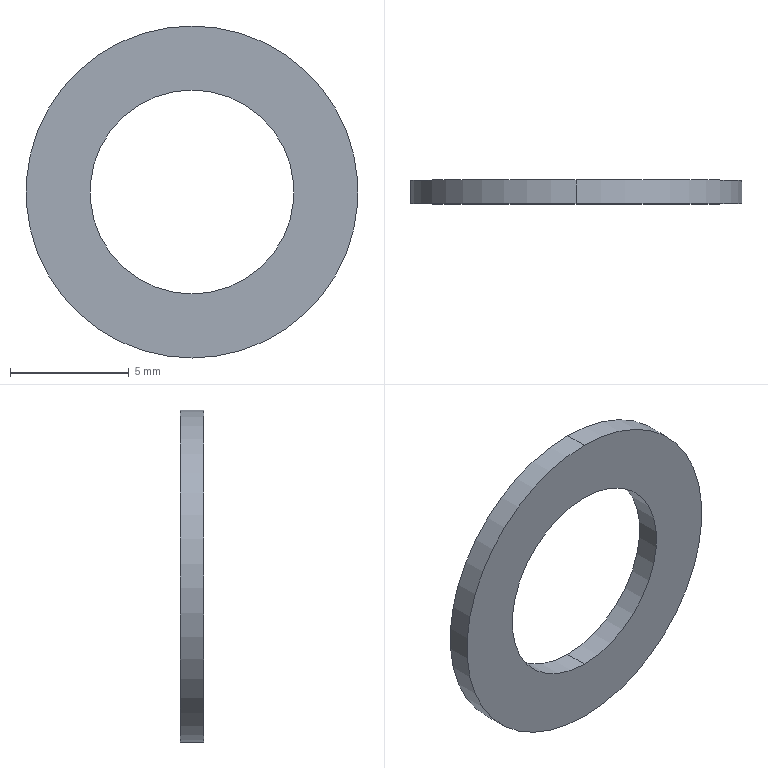Part | STEP file | Vibration plate 3-06_default | 1 solid | 6 faces | box 14 x 1 x 14 mm | volume 95.85 mm3 | cylinder 4 | plane 2 | commonest cylinder face diameters 8.6 x2 14 x2
STEP:
#1=CARTESIAN_POINT('',(0.,0.,0.));
#2=DIRECTION('',(0.,0.,1.));
#3=DIRECTION('',(1.,0.,0.));
#4=AXIS2_PLACEMENT_3D('',#1,#2,#3);
#5=CARTESIAN_POINT('',(0.,0.,4.3));
#6=VERTEX_POINT('',#5);
#7=CARTESIAN_POINT('',(0.,1.,4.3));
#8=VERTEX_POINT('',#7);
#9=CARTESIAN_POINT('',(0.,0.,4.3));
#10=DIRECTION('',(0.,1.,0.));
#11=VECTOR('',#10,1.);
#12=LINE('',#9,#11);
#13=CARTESIAN_POINT('',(0.,0.,0.));
#14=DIRECTION('',(0.,1.,0.));
#15=DIRECTION('',(0.,0.,1.));
#16=AXIS2_PLACEMENT_3D('',#13,#14,#15);
#17=CYLINDRICAL_SURFACE('',#16,4.3);
#18=CARTESIAN_POINT('',(6.283,0.));
#19=DIRECTION('',(0.,1.));
#20=VECTOR('',#19,1.);
#21=LINE('',#18,#20);
#22=(GEOMETRIC_REPRESENTATION_CONTEXT(2)PARAMETRIC_REPRESENTATION_CONTEXT()REPRESENTATION_CONTEXT('',''));
#23=DEFINITIONAL_REPRESENTATION('',(#21),#22);
#24=PCURVE('',#17,#23);
#25=CARTESIAN_POINT('',(0.,0.,0.));
#26=DIRECTION('',(0.,1.,0.));
#27=DIRECTION('',(0.,0.,1.));
#28=AXIS2_PLACEMENT_3D('',#25,#26,#27);
#29=CYLINDRICAL_SURFACE('',#28,4.3);
#30=CARTESIAN_POINT('',(0.,0.));
#31=DIRECTION('',(0.,1.));
#32=VECTOR('',#31,1.);
#33=LINE('',#30,#32);
#34=(GEOMETRIC_REPRESENTATION_CONTEXT(2)PARAMETRIC_REPRESENTATION_CONTEXT()REPRESENTATION_CONTEXT('',''));
#35=DEFINITIONAL_REPRESENTATION('',(#33),#34);
#36=PCURVE('',#29,#35);
#37=SURFACE_CURVE('',#12,(#24,#36),.PCURVE_S1.);
#38=EDGE_CURVE('',#6,#8,#37,.T.);
#39=ORIENTED_EDGE('',*,*,#38,.T.);
#40=CARTESIAN_POINT('',(0.,1.,-4.3));
#41=VERTEX_POINT('',#40);
#42=CARTESIAN_POINT('',(0.,1.,0.));
#43=DIRECTION('',(0.,-1.,0.));
#44=DIRECTION('',(0.,0.,1.));
#45=AXIS2_PLACEMENT_3D('',#42,#43,#44);
#46=CIRCLE('',#45,4.3);
#47=CARTESIAN_POINT('',(6.283,1.));
#48=DIRECTION('',(-1.,0.));
#49=VECTOR('',#48,1.);
#50=LINE('',#47,#49);
#51=(GEOMETRIC_REPRESENTATION_CONTEXT(2)PARAMETRIC_REPRESENTATION_CONTEXT()REPRESENTATION_CONTEXT('',''));
#52=DEFINITIONAL_REPRESENTATION('',(#50),#51);
#53=PCURVE('',#17,#52);
#54=CARTESIAN_POINT('',(0.,1.,0.));
#55=DIRECTION('',(0.,1.,0.));
#56=DIRECTION('',(0.,0.,1.));
#57=AXIS2_PLACEMENT_3D('',#54,#55,#56);
#58=PLANE('',#57);
#59=CARTESIAN_POINT('',(4.3,0.));
#60=CARTESIAN_POINT('',(4.3,-7.448));
#61=CARTESIAN_POINT('',(-2.15,-3.724));
#62=CARTESIAN_POINT('',(-8.6,0.));
#63=CARTESIAN_POINT('',(-2.15,3.724));
#64=CARTESIAN_POINT('',(4.3,7.448));
#65=CARTESIAN_POINT('',(4.3,0.));
#66=(BOUNDED_CURVE()B_SPLINE_CURVE(2,(#59,#60,#61,#62,#63,#64,#65),.UNSPECIFIED.,.T.,.F.)B_SPLINE_CURVE_WITH_KNOTS((1,2,2,2,2,1),(-2.094,0.,2.094,4.189,6.283,8.378),.UNSPECIFIED.)CURVE()GEOMETRIC_REPRESENTATION_ITEM()RATIONAL_B_SPLINE_CURVE((1.,0.5,1.,0.5,1.,0.5,1.))REPRESENTATION_ITEM(''));
#67=(GEOMETRIC_REPRESENTATION_CONTEXT(2)PARAMETRIC_REPRESENTATION_CONTEXT()REPRESENTATION_CONTEXT('',''));
#68=DEFINITIONAL_REPRESENTATION('',(#66),#67);
#69=PCURVE('',#58,#68);
#70=SURFACE_CURVE('',#46,(#53,#69),.PCURVE_S1.);
#71=EDGE_CURVE('',#8,#41,#70,.T.);
#72=ORIENTED_EDGE('',*,*,#71,.T.);
#73=CARTESIAN_POINT('',(0.,0.,-4.3));
#74=VERTEX_POINT('',#73);
#75=CARTESIAN_POINT('',(0.,0.,-4.3));
#76=DIRECTION('',(0.,1.,0.));
#77=VECTOR('',#76,1.);
#78=LINE('',#75,#77);
#79=CARTESIAN_POINT('',(3.142,0.));
#80=DIRECTION('',(0.,1.));
#81=VECTOR('',#80,1.);
#82=LINE('',#79,#81);
#83=(GEOMETRIC_REPRESENTATION_CONTEXT(2)PARAMETRIC_REPRESENTATION_CONTEXT()REPRESENTATION_CONTEXT('',''));
#84=DEFINITIONAL_REPRESENTATION('',(#82),#83);
#85=PCURVE('',#17,#84);
#86=CARTESIAN_POINT('',(3.142,0.));
#87=DIRECTION('',(0.,1.));
#88=VECTOR('',#87,1.);
#89=LINE('',#86,#88);
#90=(GEOMETRIC_REPRESENTATION_CONTEXT(2)PARAMETRIC_REPRESENTATION_CONTEXT()REPRESENTATION_CONTEXT('',''));
#91=DEFINITIONAL_REPRESENTATION('',(#89),#90);
#92=PCURVE('',#29,#91);
#93=SURFACE_CURVE('',#78,(#85,#92),.PCURVE_S1.);
#94=EDGE_CURVE('',#74,#41,#93,.T.);
#95=ORIENTED_EDGE('',*,*,#94,.F.);
#96=CARTESIAN_POINT('',(0.,0.,0.));
#97=DIRECTION('',(0.,-1.,0.));
#98=DIRECTION('',(0.,0.,1.));
#99=AXIS2_PLACEMENT_3D('',#96,#97,#98);
#100=CIRCLE('',#99,4.3);
#101=CARTESIAN_POINT('',(6.283,0.));
#102=DIRECTION('',(-1.,0.));
#103=VECTOR('',#102,1.);
#104=LINE('',#101,#103);
#105=(GEOMETRIC_REPRESENTATION_CONTEXT(2)PARAMETRIC_REPRESENTATION_CONTEXT()REPRESENTATION_CONTEXT('',''));
#106=DEFINITIONAL_REPRESENTATION('',(#104),#105);
#107=PCURVE('',#17,#106);
#108=CARTESIAN_POINT('',(0.,0.,0.));
#109=DIRECTION('',(0.,1.,0.));
#110=DIRECTION('',(0.,0.,1.));
#111=AXIS2_PLACEMENT_3D('',#108,#109,#110);
#112=PLANE('',#111);
#113=CARTESIAN_POINT('',(4.3,0.));
#114=CARTESIAN_POINT('',(4.3,-7.448));
#115=CARTESIAN_POINT('',(-2.15,-3.724));
#116=CARTESIAN_POINT('',(-8.6,0.));
#117=CARTESIAN_POINT('',(-2.15,3.724));
#118=CARTESIAN_POINT('',(4.3,7.448));
#119=CARTESIAN_POINT('',(4.3,0.));
#120=(BOUNDED_CURVE()B_SPLINE_CURVE(2,(#113,#114,#115,#116,#117,#118,#119),.UNSPECIFIED.,.T.,.F.)B_SPLINE_CURVE_WITH_KNOTS((1,2,2,2,2,1),(-2.094,0.,2.094,4.189,6.283,8.378),.UNSPECIFIED.)CURVE()GEOMETRIC_REPRESENTATION_ITEM()RATIONAL_B_SPLINE_CURVE((1.,0.5,1.,0.5,1.,0.5,1.))REPRESENTATION_ITEM(''));
#121=(GEOMETRIC_REPRESENTATION_CONTEXT(2)PARAMETRIC_REPRESENTATION_CONTEXT()REPRESENTATION_CONTEXT('',''));
#122=DEFINITIONAL_REPRESENTATION('',(#120),#121);
#123=PCURVE('',#112,#122);
#124=SURFACE_CURVE('',#100,(#107,#123),.PCURVE_S1.);
#125=EDGE_CURVE('',#6,#74,#124,.T.);
#126=ORIENTED_EDGE('',*,*,#125,.F.);
#127=EDGE_LOOP('',(#39,#72,#95,#126));
#128=FACE_BOUND('',#127,.F.);
#129=ADVANCED_FACE('',(#128),#17,.F.);
#130=CARTESIAN_POINT('',(0.,0.,7.));
#131=VERTEX_POINT('',#130);
#132=CARTESIAN_POINT('',(0.,0.,-7.));
#133=VERTEX_POINT('',#132);
#134=CARTESIAN_POINT('',(0.,0.,0.));
#135=DIRECTION('',(0.,1.,0.));
#136=DIRECTION('',(0.,0.,1.));
#137=AXIS2_PLACEMENT_3D('',#134,#135,#136);
#138=CIRCLE('',#137,7.);
#139=CARTESIAN_POINT('',(0.,0.,0.));
#140=DIRECTION('',(0.,1.,0.));
#141=DIRECTION('',(0.,0.,1.));
#142=AXIS2_PLACEMENT_3D('',#139,#140,#141);
#143=CYLINDRICAL_SURFACE('',#142,7.);
#144=CARTESIAN_POINT('',(0.,0.));
#145=DIRECTION('',(1.,0.));
#146=VECTOR('',#145,1.);
#147=LINE('',#144,#146);
#148=(GEOMETRIC_REPRESENTATION_CONTEXT(2)PARAMETRIC_REPRESENTATION_CONTEXT()REPRESENTATION_CONTEXT('',''));
#149=DEFINITIONAL_REPRESENTATION('',(#147),#148);
#150=PCURVE('',#143,#149);
#151=CARTESIAN_POINT('',(0.,0.));
#152=DIRECTION('',(1.,0.));
#153=AXIS2_PLACEMENT_2D('',#151,#152);
#154=CIRCLE('',#153,7.);
#155=(GEOMETRIC_REPRESENTATION_CONTEXT(2)PARAMETRIC_REPRESENTATION_CONTEXT()REPRESENTATION_CONTEXT('',''));
#156=DEFINITIONAL_REPRESENTATION('',(#154),#155);
#157=PCURVE('',#112,#156);
#158=SURFACE_CURVE('',#138,(#150,#157),.PCURVE_S1.);
#159=EDGE_CURVE('',#131,#133,#158,.T.);
#160=ORIENTED_EDGE('',*,*,#159,.T.);
#161=CARTESIAN_POINT('',(0.,1.,-7.));
#162=VERTEX_POINT('',#161);
#163=CARTESIAN_POINT('',(0.,0.,-7.));
#164=DIRECTION('',(0.,1.,0.));
#165=VECTOR('',#164,1.);
#166=LINE('',#163,#165);
#167=CARTESIAN_POINT('',(3.142,0.));
#168=DIRECTION('',(0.,1.));
#169=VECTOR('',#168,1.);
#170=LINE('',#167,#169);
#171=(GEOMETRIC_REPRESENTATION_CONTEXT(2)PARAMETRIC_REPRESENTATION_CONTEXT()REPRESENTATION_CONTEXT('',''));
#172=DEFINITIONAL_REPRESENTATION('',(#170),#171);
#173=PCURVE('',#143,#172);
#174=CARTESIAN_POINT('',(0.,0.,0.));
#175=DIRECTION('',(0.,1.,0.));
#176=DIRECTION('',(0.,0.,1.));
#177=AXIS2_PLACEMENT_3D('',#174,#175,#176);
#178=CYLINDRICAL_SURFACE('',#177,7.);
#179=CARTESIAN_POINT('',(3.142,0.));
#180=DIRECTION('',(0.,1.));
#181=VECTOR('',#180,1.);
#182=LINE('',#179,#181);
#183=(GEOMETRIC_REPRESENTATION_CONTEXT(2)PARAMETRIC_REPRESENTATION_CONTEXT()REPRESENTATION_CONTEXT('',''));
#184=DEFINITIONAL_REPRESENTATION('',(#182),#183);
#185=PCURVE('',#178,#184);
#186=SURFACE_CURVE('',#166,(#173,#185),.PCURVE_S1.);
#187=EDGE_CURVE('',#133,#162,#186,.T.);
#188=ORIENTED_EDGE('',*,*,#187,.T.);
#189=CARTESIAN_POINT('',(0.,1.,7.));
#190=VERTEX_POINT('',#189);
#191=CARTESIAN_POINT('',(0.,1.,0.));
#192=DIRECTION('',(0.,-1.,0.));
#193=DIRECTION('',(0.,0.,1.));
#194=AXIS2_PLACEMENT_3D('',#191,#192,#193);
#195=CIRCLE('',#194,7.);
#196=CARTESIAN_POINT('',(6.283,1.));
#197=DIRECTION('',(-1.,0.));
#198=VECTOR('',#197,1.);
#199=LINE('',#196,#198);
#200=(GEOMETRIC_REPRESENTATION_CONTEXT(2)PARAMETRIC_REPRESENTATION_CONTEXT()REPRESENTATION_CONTEXT('',''));
#201=DEFINITIONAL_REPRESENTATION('',(#199),#200);
#202=PCURVE('',#143,#201);
#203=CARTESIAN_POINT('',(7.,0.));
#204=CARTESIAN_POINT('',(7.,-12.124));
#205=CARTESIAN_POINT('',(-3.5,-6.062));
#206=CARTESIAN_POINT('',(-14.,0.));
#207=CARTESIAN_POINT('',(-3.5,6.062));
#208=CARTESIAN_POINT('',(7.,12.124));
#209=CARTESIAN_POINT('',(7.,0.));
#210=(BOUNDED_CURVE()B_SPLINE_CURVE(2,(#203,#204,#205,#206,#207,#208,#209),.UNSPECIFIED.,.T.,.F.)B_SPLINE_CURVE_WITH_KNOTS((1,2,2,2,2,1),(-2.094,0.,2.094,4.189,6.283,8.378),.UNSPECIFIED.)CURVE()GEOMETRIC_REPRESENTATION_ITEM()RATIONAL_B_SPLINE_CURVE((1.,0.5,1.,0.5,1.,0.5,1.))REPRESENTATION_ITEM(''));
#211=(GEOMETRIC_REPRESENTATION_CONTEXT(2)PARAMETRIC_REPRESENTATION_CONTEXT()REPRESENTATION_CONTEXT('',''));
#212=DEFINITIONAL_REPRESENTATION('',(#210),#211);
#213=PCURVE('',#58,#212);
#214=SURFACE_CURVE('',#195,(#202,#213),.PCURVE_S1.);
#215=EDGE_CURVE('',#162,#190,#214,.T.);
#216=ORIENTED_EDGE('',*,*,#215,.T.);
#217=CARTESIAN_POINT('',(0.,0.,7.));
#218=DIRECTION('',(0.,1.,0.));
#219=VECTOR('',#218,1.);
#220=LINE('',#217,#219);
#221=CARTESIAN_POINT('',(0.,0.));
#222=DIRECTION('',(0.,1.));
#223=VECTOR('',#222,1.);
#224=LINE('',#221,#223);
#225=(GEOMETRIC_REPRESENTATION_CONTEXT(2)PARAMETRIC_REPRESENTATION_CONTEXT()REPRESENTATION_CONTEXT('',''));
#226=DEFINITIONAL_REPRESENTATION('',(#224),#225);
#227=PCURVE('',#143,#226);
#228=CARTESIAN_POINT('',(6.283,0.));
#229=DIRECTION('',(0.,1.));
#230=VECTOR('',#229,1.);
#231=LINE('',#228,#230);
#232=(GEOMETRIC_REPRESENTATION_CONTEXT(2)PARAMETRIC_REPRESENTATION_CONTEXT()REPRESENTATION_CONTEXT('',''));
#233=DEFINITIONAL_REPRESENTATION('',(#231),#232);
#234=PCURVE('',#178,#233);
#235=SURFACE_CURVE('',#220,(#227,#234),.PCURVE_S1.);
#236=EDGE_CURVE('',#131,#190,#235,.T.);
#237=ORIENTED_EDGE('',*,*,#236,.F.);
#238=EDGE_LOOP('',(#160,#188,#216,#237));
#239=FACE_BOUND('',#238,.T.);
#240=ADVANCED_FACE('',(#239),#143,.T.);
#241=ORIENTED_EDGE('',*,*,#125,.F.);
#242=CARTESIAN_POINT('',(0.,0.,0.));
#243=DIRECTION('',(0.,-1.,0.));
#244=DIRECTION('',(0.,0.,1.));
#245=AXIS2_PLACEMENT_3D('',#242,#243,#244);
#246=CIRCLE('',#245,4.3);
#247=CARTESIAN_POINT('',(4.3,0.));
#248=CARTESIAN_POINT('',(4.3,-7.448));
#249=CARTESIAN_POINT('',(-2.15,-3.724));
#250=CARTESIAN_POINT('',(-8.6,0.));
#251=CARTESIAN_POINT('',(-2.15,3.724));
#252=CARTESIAN_POINT('',(4.3,7.448));
#253=CARTESIAN_POINT('',(4.3,0.));
#254=(BOUNDED_CURVE()B_SPLINE_CURVE(2,(#247,#248,#249,#250,#251,#252,#253),.UNSPECIFIED.,.T.,.F.)B_SPLINE_CURVE_WITH_KNOTS((1,2,2,2,2,1),(-2.094,0.,2.094,4.189,6.283,8.378),.UNSPECIFIED.)CURVE()GEOMETRIC_REPRESENTATION_ITEM()RATIONAL_B_SPLINE_CURVE((1.,0.5,1.,0.5,1.,0.5,1.))REPRESENTATION_ITEM(''));
#255=(GEOMETRIC_REPRESENTATION_CONTEXT(2)PARAMETRIC_REPRESENTATION_CONTEXT()REPRESENTATION_CONTEXT('',''));
#256=DEFINITIONAL_REPRESENTATION('',(#254),#255);
#257=PCURVE('',#112,#256);
#258=CARTESIAN_POINT('',(6.283,0.));
#259=DIRECTION('',(-1.,0.));
#260=VECTOR('',#259,1.);
#261=LINE('',#258,#260);
#262=(GEOMETRIC_REPRESENTATION_CONTEXT(2)PARAMETRIC_REPRESENTATION_CONTEXT()REPRESENTATION_CONTEXT('',''));
#263=DEFINITIONAL_REPRESENTATION('',(#261),#262);
#264=PCURVE('',#29,#263);
#265=SURFACE_CURVE('',#246,(#257,#264),.PCURVE_S1.);
#266=EDGE_CURVE('',#74,#6,#265,.T.);
#267=ORIENTED_EDGE('',*,*,#266,.F.);
#268=EDGE_LOOP('',(#241,#267));
#269=FACE_BOUND('',#268,.T.);
#270=ORIENTED_EDGE('',*,*,#159,.F.);
#271=CARTESIAN_POINT('',(0.,0.,0.));
#272=DIRECTION('',(0.,1.,0.));
#273=DIRECTION('',(0.,0.,1.));
#274=AXIS2_PLACEMENT_3D('',#271,#272,#273);
#275=CIRCLE('',#274,7.);
#276=CARTESIAN_POINT('',(0.,0.));
#277=DIRECTION('',(1.,0.));
#278=AXIS2_PLACEMENT_2D('',#276,#277);
#279=CIRCLE('',#278,7.);
#280=(GEOMETRIC_REPRESENTATION_CONTEXT(2)PARAMETRIC_REPRESENTATION_CONTEXT()REPRESENTATION_CONTEXT('',''));
#281=DEFINITIONAL_REPRESENTATION('',(#279),#280);
#282=PCURVE('',#112,#281);
#283=CARTESIAN_POINT('',(0.,0.));
#284=DIRECTION('',(1.,0.));
#285=VECTOR('',#284,1.);
#286=LINE('',#283,#285);
#287=(GEOMETRIC_REPRESENTATION_CONTEXT(2)PARAMETRIC_REPRESENTATION_CONTEXT()REPRESENTATION_CONTEXT('',''));
#288=DEFINITIONAL_REPRESENTATION('',(#286),#287);
#289=PCURVE('',#178,#288);
#290=SURFACE_CURVE('',#275,(#282,#289),.PCURVE_S1.);
#291=EDGE_CURVE('',#133,#131,#290,.T.);
#292=ORIENTED_EDGE('',*,*,#291,.F.);
#293=EDGE_LOOP('',(#270,#292));
#294=FACE_BOUND('',#293,.T.);
#295=ADVANCED_FACE('',(#269,#294),#112,.F.);
#296=CARTESIAN_POINT('',(0.,1.,0.));
#297=DIRECTION('',(0.,-1.,0.));
#298=DIRECTION('',(0.,0.,1.));
#299=AXIS2_PLACEMENT_3D('',#296,#297,#298);
#300=CIRCLE('',#299,4.3);
#301=CARTESIAN_POINT('',(6.283,1.));
#302=DIRECTION('',(-1.,0.));
#303=VECTOR('',#302,1.);
#304=LINE('',#301,#303);
#305=(GEOMETRIC_REPRESENTATION_CONTEXT(2)PARAMETRIC_REPRESENTATION_CONTEXT()REPRESENTATION_CONTEXT('',''));
#306=DEFINITIONAL_REPRESENTATION('',(#304),#305);
#307=PCURVE('',#29,#306);
#308=CARTESIAN_POINT('',(4.3,0.));
#309=CARTESIAN_POINT('',(4.3,-7.448));
#310=CARTESIAN_POINT('',(-2.15,-3.724));
#311=CARTESIAN_POINT('',(-8.6,0.));
#312=CARTESIAN_POINT('',(-2.15,3.724));
#313=CARTESIAN_POINT('',(4.3,7.448));
#314=CARTESIAN_POINT('',(4.3,0.));
#315=(BOUNDED_CURVE()B_SPLINE_CURVE(2,(#308,#309,#310,#311,#312,#313,#314),.UNSPECIFIED.,.T.,.F.)B_SPLINE_CURVE_WITH_KNOTS((1,2,2,2,2,1),(-2.094,0.,2.094,4.189,6.283,8.378),.UNSPECIFIED.)CURVE()GEOMETRIC_REPRESENTATION_ITEM()RATIONAL_B_SPLINE_CURVE((1.,0.5,1.,0.5,1.,0.5,1.))REPRESENTATION_ITEM(''));
#316=(GEOMETRIC_REPRESENTATION_CONTEXT(2)PARAMETRIC_REPRESENTATION_CONTEXT()REPRESENTATION_CONTEXT('',''));
#317=DEFINITIONAL_REPRESENTATION('',(#315),#316);
#318=PCURVE('',#58,#317);
#319=SURFACE_CURVE('',#300,(#307,#318),.PCURVE_S1.);
#320=EDGE_CURVE('',#41,#8,#319,.T.);
#321=ORIENTED_EDGE('',*,*,#320,.T.);
#322=ORIENTED_EDGE('',*,*,#38,.F.);
#323=ORIENTED_EDGE('',*,*,#266,.F.);
#324=ORIENTED_EDGE('',*,*,#94,.T.);
#325=EDGE_LOOP('',(#321,#322,#323,#324));
#326=FACE_BOUND('',#325,.F.);
#327=ADVANCED_FACE('',(#326),#29,.F.);
#328=ORIENTED_EDGE('',*,*,#187,.F.);
#329=ORIENTED_EDGE('',*,*,#291,.T.);
#330=ORIENTED_EDGE('',*,*,#236,.T.);
#331=CARTESIAN_POINT('',(0.,1.,0.));
#332=DIRECTION('',(0.,-1.,0.));
#333=DIRECTION('',(0.,0.,1.));
#334=AXIS2_PLACEMENT_3D('',#331,#332,#333);
#335=CIRCLE('',#334,7.);
#336=CARTESIAN_POINT('',(6.283,1.));
#337=DIRECTION('',(-1.,0.));
#338=VECTOR('',#337,1.);
#339=LINE('',#336,#338);
#340=(GEOMETRIC_REPRESENTATION_CONTEXT(2)PARAMETRIC_REPRESENTATION_CONTEXT()REPRESENTATION_CONTEXT('',''));
#341=DEFINITIONAL_REPRESENTATION('',(#339),#340);
#342=PCURVE('',#178,#341);
#343=CARTESIAN_POINT('',(7.,0.));
#344=CARTESIAN_POINT('',(7.,-12.124));
#345=CARTESIAN_POINT('',(-3.5,-6.062));
#346=CARTESIAN_POINT('',(-14.,0.));
#347=CARTESIAN_POINT('',(-3.5,6.062));
#348=CARTESIAN_POINT('',(7.,12.124));
#349=CARTESIAN_POINT('',(7.,0.));
#350=(BOUNDED_CURVE()B_SPLINE_CURVE(2,(#343,#344,#345,#346,#347,#348,#349),.UNSPECIFIED.,.T.,.F.)B_SPLINE_CURVE_WITH_KNOTS((1,2,2,2,2,1),(-2.094,0.,2.094,4.189,6.283,8.378),.UNSPECIFIED.)CURVE()GEOMETRIC_REPRESENTATION_ITEM()RATIONAL_B_SPLINE_CURVE((1.,0.5,1.,0.5,1.,0.5,1.))REPRESENTATION_ITEM(''));
#351=(GEOMETRIC_REPRESENTATION_CONTEXT(2)PARAMETRIC_REPRESENTATION_CONTEXT()REPRESENTATION_CONTEXT('',''));
#352=DEFINITIONAL_REPRESENTATION('',(#350),#351);
#353=PCURVE('',#58,#352);
#354=SURFACE_CURVE('',#335,(#342,#353),.PCURVE_S1.);
#355=EDGE_CURVE('',#190,#162,#354,.T.);
#356=ORIENTED_EDGE('',*,*,#355,.T.);
#357=EDGE_LOOP('',(#328,#329,#330,#356));
#358=FACE_BOUND('',#357,.T.);
#359=ADVANCED_FACE('',(#358),#178,.T.);
#360=ORIENTED_EDGE('',*,*,#71,.T.);
#361=ORIENTED_EDGE('',*,*,#320,.T.);
#362=EDGE_LOOP('',(#360,#361));
#363=FACE_BOUND('',#362,.T.);
#364=ORIENTED_EDGE('',*,*,#355,.F.);
#365=ORIENTED_EDGE('',*,*,#215,.F.);
#366=EDGE_LOOP('',(#364,#365));
#367=FACE_BOUND('',#366,.T.);
#368=ADVANCED_FACE('',(#363,#367),#58,.T.);
#369=CLOSED_SHELL('',(#129,#240,#295,#327,#359,#368));
#370=MANIFOLD_SOLID_BREP('',#369);
#371=(LENGTH_UNIT()NAMED_UNIT(*)SI_UNIT(.MILLI.,.METRE.));
#372=UNCERTAINTY_MEASURE_WITH_UNIT(LENGTH_MEASURE(0.0000001),#371,'','');
#373=(NAMED_UNIT(*)PLANE_ANGLE_UNIT()SI_UNIT($,.RADIAN.));
#374=(NAMED_UNIT(*)SI_UNIT($,.STERADIAN.)SOLID_ANGLE_UNIT());
#375=(GEOMETRIC_REPRESENTATION_CONTEXT(3)GLOBAL_UNCERTAINTY_ASSIGNED_CONTEXT((#372))GLOBAL_UNIT_ASSIGNED_CONTEXT((#371,#373,#374))REPRESENTATION_CONTEXT('',''));
#376=ADVANCED_BREP_SHAPE_REPRESENTATION('',(#4,#370),#375);